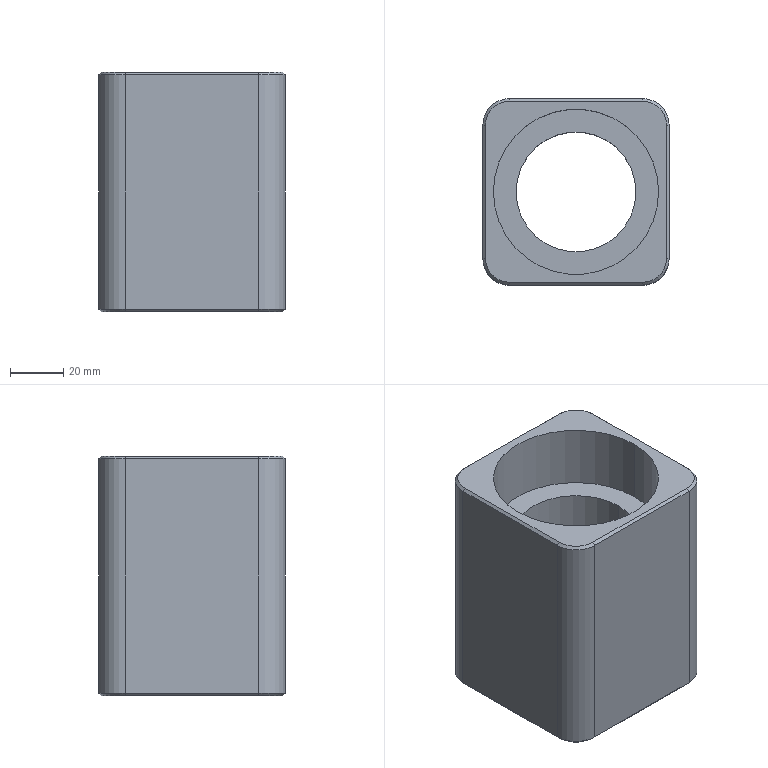Part | STEP file | MILLED_BLOCK_FOR_AXISV11 | 1 solid | 34 faces | box 70 x 70 x 90 mm | volume 221300 mm3 | plane 16 | cylinder 10 | cone 8 | commonest cylinder face diameters 20 x4 62 x4 45 x2